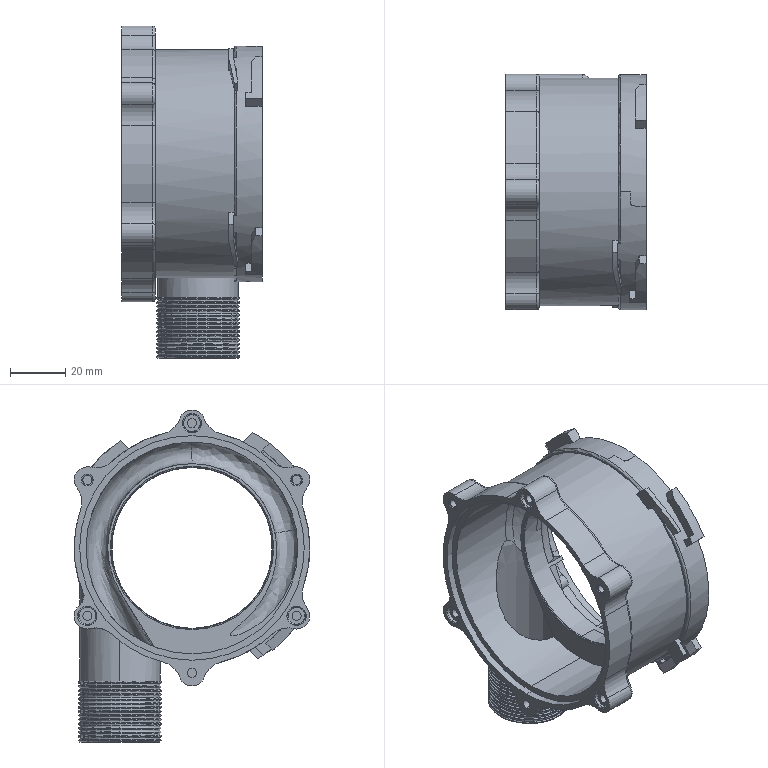Part | STEP file | 8_20_3_1_1_14 | 1 solid | 436 faces | box 50.6 x 85 x 119.75 mm | volume 65552 mm3 | cylinder 129 | torus 115 | plane 99 | spline 57 | cone 34 | other 2 | commonest cylinder face diameters 29 x32 76.2 x16 5 x14 3.3 x12 16 x11 85 x8